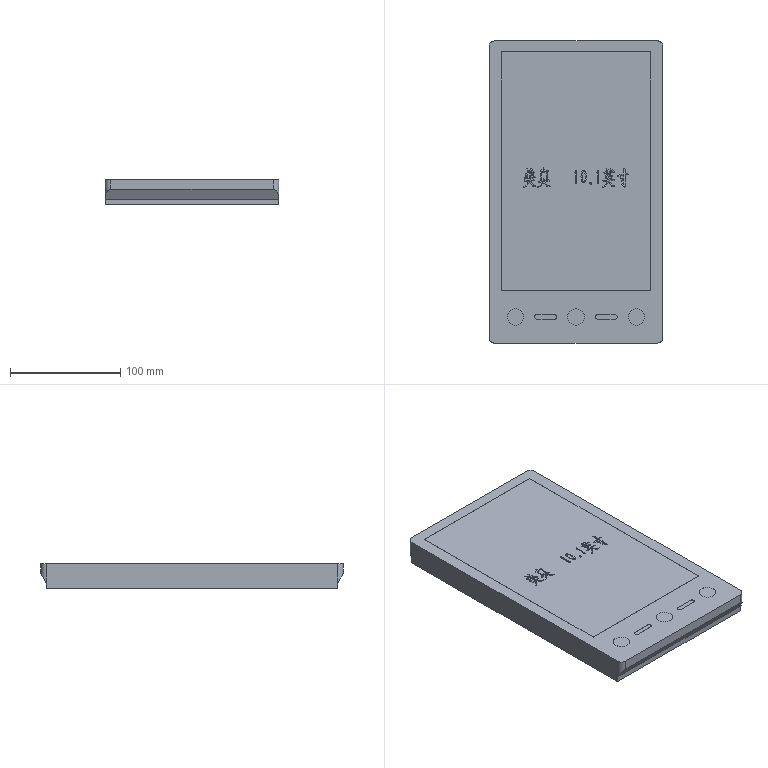Part | 1 solid | 400 faces | box 157.5 x 274 x 23 mm | volume 971918 mm3 | plane 274 | spline 110 | cylinder 16 | commonest cylinder face diameters 4 x6 15 x6 10 x4